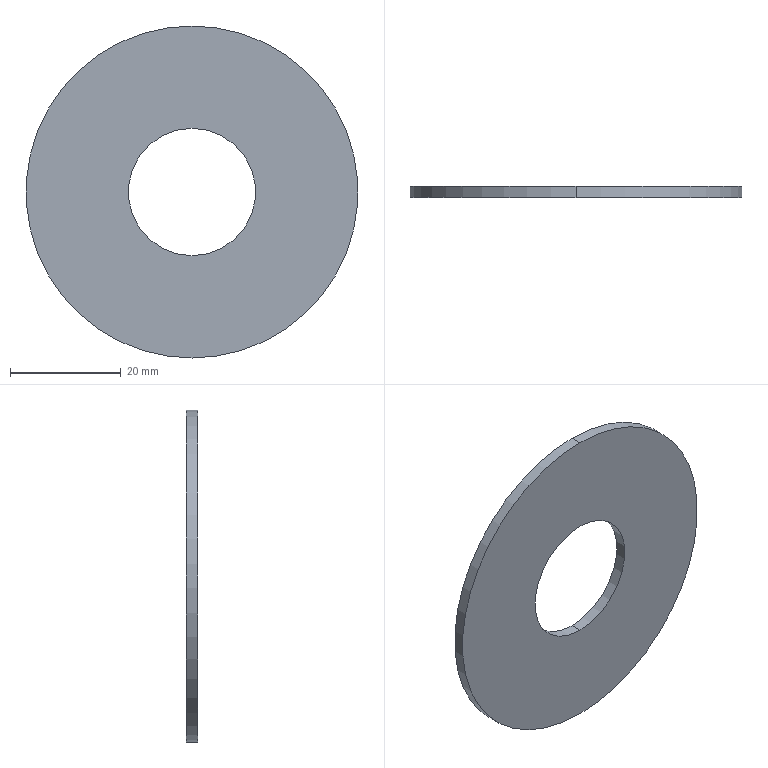Part | SolidWorks | features Extrusion 1 | 1 solid | 6 faces | box 60 x 2 x 60 mm | volume 4824 mm3 | cylinder 4 | plane 2 | commonest cylinder face diameters 23 x2 60 x2
STEP:
#1=CARTESIAN_POINT('',(0.,2.,-11.5));
#2=VERTEX_POINT('',#1);
#3=CARTESIAN_POINT('',(0.,2.,11.5));
#4=VERTEX_POINT('',#3);
#5=CARTESIAN_POINT('',(0.,2.,0.));
#6=DIRECTION('',(0.,1.,0.));
#7=DIRECTION('',(0.,0.,1.));
#8=AXIS2_PLACEMENT_3D('',#5,#6,#7);
#9=CIRCLE('',#8,11.5);
#10=EDGE_CURVE('',#2,#4,#9,.T.);
#11=ORIENTED_EDGE('',*,*,#10,.T.);
#12=CARTESIAN_POINT('',(0.,0.,11.5));
#13=VERTEX_POINT('',#12);
#14=CARTESIAN_POINT('',(0.,2.,11.5));
#15=DIRECTION('',(0.,-1.,0.));
#16=VECTOR('',#15,1000.);
#17=LINE('',#14,#16);
#18=EDGE_CURVE('',#4,#13,#17,.T.);
#19=ORIENTED_EDGE('',*,*,#18,.T.);
#20=CARTESIAN_POINT('',(0.,0.,-11.5));
#21=VERTEX_POINT('',#20);
#22=CARTESIAN_POINT('',(0.,0.,0.));
#23=DIRECTION('',(0.,1.,0.));
#24=DIRECTION('',(0.,0.,1.));
#25=AXIS2_PLACEMENT_3D('',#22,#23,#24);
#26=CIRCLE('',#25,11.5);
#27=EDGE_CURVE('',#21,#13,#26,.T.);
#28=ORIENTED_EDGE('',*,*,#27,.F.);
#29=CARTESIAN_POINT('',(0.,2.,-11.5));
#30=DIRECTION('',(0.,-1.,0.));
#31=VECTOR('',#30,1000.);
#32=LINE('',#29,#31);
#33=EDGE_CURVE('',#2,#21,#32,.T.);
#34=ORIENTED_EDGE('',*,*,#33,.F.);
#35=EDGE_LOOP('',(#11,#19,#28,#34));
#36=FACE_OUTER_BOUND('',#35,.T.);
#37=CARTESIAN_POINT('',(0.,2.,0.));
#38=DIRECTION('',(0.,-1.,0.));
#39=DIRECTION('',(0.,0.,-1.));
#40=AXIS2_PLACEMENT_3D('',#37,#38,#39);
#41=CYLINDRICAL_SURFACE('',#40,11.5);
#42=ADVANCED_FACE('',(#36),#41,.F.);
#43=CARTESIAN_POINT('',(0.,2.,30.));
#44=VERTEX_POINT('',#43);
#45=CARTESIAN_POINT('',(0.,2.,-30.));
#46=VERTEX_POINT('',#45);
#47=CARTESIAN_POINT('',(0.,2.,0.));
#48=DIRECTION('',(0.,1.,0.));
#49=DIRECTION('',(0.,0.,1.));
#50=AXIS2_PLACEMENT_3D('',#47,#48,#49);
#51=CIRCLE('',#50,30.);
#52=EDGE_CURVE('',#44,#46,#51,.T.);
#53=ORIENTED_EDGE('',*,*,#52,.F.);
#54=CARTESIAN_POINT('',(0.,0.,30.));
#55=VERTEX_POINT('',#54);
#56=CARTESIAN_POINT('',(0.,2.,30.));
#57=DIRECTION('',(0.,-1.,0.));
#58=VECTOR('',#57,1000.);
#59=LINE('',#56,#58);
#60=EDGE_CURVE('',#44,#55,#59,.T.);
#61=ORIENTED_EDGE('',*,*,#60,.T.);
#62=CARTESIAN_POINT('',(0.,0.,-30.));
#63=VERTEX_POINT('',#62);
#64=CARTESIAN_POINT('',(0.,0.,0.));
#65=DIRECTION('',(0.,1.,0.));
#66=DIRECTION('',(0.,0.,1.));
#67=AXIS2_PLACEMENT_3D('',#64,#65,#66);
#68=CIRCLE('',#67,30.);
#69=EDGE_CURVE('',#55,#63,#68,.T.);
#70=ORIENTED_EDGE('',*,*,#69,.T.);
#71=CARTESIAN_POINT('',(0.,2.,-30.));
#72=DIRECTION('',(0.,-1.,0.));
#73=VECTOR('',#72,1000.);
#74=LINE('',#71,#73);
#75=EDGE_CURVE('',#46,#63,#74,.T.);
#76=ORIENTED_EDGE('',*,*,#75,.F.);
#77=EDGE_LOOP('',(#53,#61,#70,#76));
#78=FACE_OUTER_BOUND('',#77,.T.);
#79=CARTESIAN_POINT('',(0.,2.,0.));
#80=DIRECTION('',(0.,-1.,0.));
#81=DIRECTION('',(0.,0.,-1.));
#82=AXIS2_PLACEMENT_3D('',#79,#80,#81);
#83=CYLINDRICAL_SURFACE('',#82,30.);
#84=ADVANCED_FACE('',(#78),#83,.T.);
#85=CARTESIAN_POINT('',(0.,2.,0.));
#86=DIRECTION('',(0.,1.,0.));
#87=DIRECTION('',(0.,0.,1.));
#88=AXIS2_PLACEMENT_3D('',#85,#86,#87);
#89=CIRCLE('',#88,30.);
#90=EDGE_CURVE('',#46,#44,#89,.T.);
#91=ORIENTED_EDGE('',*,*,#90,.T.);
#92=ORIENTED_EDGE('',*,*,#52,.T.);
#93=EDGE_LOOP('',(#91,#92));
#94=FACE_OUTER_BOUND('',#93,.T.);
#95=ORIENTED_EDGE('',*,*,#10,.F.);
#96=CARTESIAN_POINT('',(0.,2.,0.));
#97=DIRECTION('',(0.,1.,0.));
#98=DIRECTION('',(0.,0.,1.));
#99=AXIS2_PLACEMENT_3D('',#96,#97,#98);
#100=CIRCLE('',#99,11.5);
#101=EDGE_CURVE('',#4,#2,#100,.T.);
#102=ORIENTED_EDGE('',*,*,#101,.F.);
#103=EDGE_LOOP('',(#95,#102));
#104=FACE_BOUND('',#103,.T.);
#105=CARTESIAN_POINT('',(0.,2.,0.));
#106=DIRECTION('',(0.,1.,0.));
#107=DIRECTION('',(0.,0.,1.));
#108=AXIS2_PLACEMENT_3D('',#105,#106,#107);
#109=PLANE('',#108);
#110=ADVANCED_FACE('',(#94,#104),#109,.T.);
#111=CARTESIAN_POINT('',(0.,0.,0.));
#112=DIRECTION('',(0.,1.,0.));
#113=DIRECTION('',(0.,0.,1.));
#114=AXIS2_PLACEMENT_3D('',#111,#112,#113);
#115=CIRCLE('',#114,30.);
#116=EDGE_CURVE('',#63,#55,#115,.T.);
#117=ORIENTED_EDGE('',*,*,#116,.F.);
#118=ORIENTED_EDGE('',*,*,#69,.F.);
#119=EDGE_LOOP('',(#117,#118));
#120=FACE_OUTER_BOUND('',#119,.T.);
#121=ORIENTED_EDGE('',*,*,#27,.T.);
#122=CARTESIAN_POINT('',(0.,0.,0.));
#123=DIRECTION('',(0.,1.,0.));
#124=DIRECTION('',(0.,0.,1.));
#125=AXIS2_PLACEMENT_3D('',#122,#123,#124);
#126=CIRCLE('',#125,11.5);
#127=EDGE_CURVE('',#13,#21,#126,.T.);
#128=ORIENTED_EDGE('',*,*,#127,.T.);
#129=EDGE_LOOP('',(#121,#128));
#130=FACE_BOUND('',#129,.T.);
#131=CARTESIAN_POINT('',(0.,0.,0.));
#132=DIRECTION('',(0.,1.,0.));
#133=DIRECTION('',(0.,0.,1.));
#134=AXIS2_PLACEMENT_3D('',#131,#132,#133);
#135=PLANE('',#134);
#136=ADVANCED_FACE('',(#120,#130),#135,.F.);
#137=ORIENTED_EDGE('',*,*,#60,.F.);
#138=ORIENTED_EDGE('',*,*,#90,.F.);
#139=ORIENTED_EDGE('',*,*,#75,.T.);
#140=ORIENTED_EDGE('',*,*,#116,.T.);
#141=EDGE_LOOP('',(#137,#138,#139,#140));
#142=FACE_OUTER_BOUND('',#141,.T.);
#143=CARTESIAN_POINT('',(0.,2.,0.));
#144=DIRECTION('',(0.,-1.,0.));
#145=DIRECTION('',(0.,0.,-1.));
#146=AXIS2_PLACEMENT_3D('',#143,#144,#145);
#147=CYLINDRICAL_SURFACE('',#146,30.);
#148=ADVANCED_FACE('',(#142),#147,.T.);
#149=ORIENTED_EDGE('',*,*,#18,.F.);
#150=ORIENTED_EDGE('',*,*,#101,.T.);
#151=ORIENTED_EDGE('',*,*,#33,.T.);
#152=ORIENTED_EDGE('',*,*,#127,.F.);
#153=EDGE_LOOP('',(#149,#150,#151,#152));
#154=FACE_OUTER_BOUND('',#153,.T.);
#155=CARTESIAN_POINT('',(0.,2.,0.));
#156=DIRECTION('',(0.,-1.,0.));
#157=DIRECTION('',(0.,0.,-1.));
#158=AXIS2_PLACEMENT_3D('',#155,#156,#157);
#159=CYLINDRICAL_SURFACE('',#158,11.5);
#160=ADVANCED_FACE('',(#154),#159,.F.);
#161=CLOSED_SHELL('',(#42,#84,#110,#136,#148,#160));
#162=MANIFOLD_SOLID_BREP('',#161);
#163=CARTESIAN_POINT('',(0.,0.,0.));
#164=DIRECTION('',(0.,0.,1.));
#165=DIRECTION('',(1.,0.,0.));
#166=AXIS2_PLACEMENT_3D('',#163,#164,#165);
#167=(LENGTH_UNIT()NAMED_UNIT(*)SI_UNIT(.MILLI.,.METRE.));
#168=UNCERTAINTY_MEASURE_WITH_UNIT(LENGTH_MEASURE(0.00001),#167,'','');
#169=(NAMED_UNIT(*)PLANE_ANGLE_UNIT()SI_UNIT($,.RADIAN.));
#170=(NAMED_UNIT(*)SI_UNIT($,.STERADIAN.)SOLID_ANGLE_UNIT());
#171=(GEOMETRIC_REPRESENTATION_CONTEXT(3)GLOBAL_UNCERTAINTY_ASSIGNED_CONTEXT((#168))GLOBAL_UNIT_ASSIGNED_CONTEXT((#167,#169,#170))REPRESENTATION_CONTEXT('',''));
#172=ADVANCED_BREP_SHAPE_REPRESENTATION('',(#162,#166),#171);